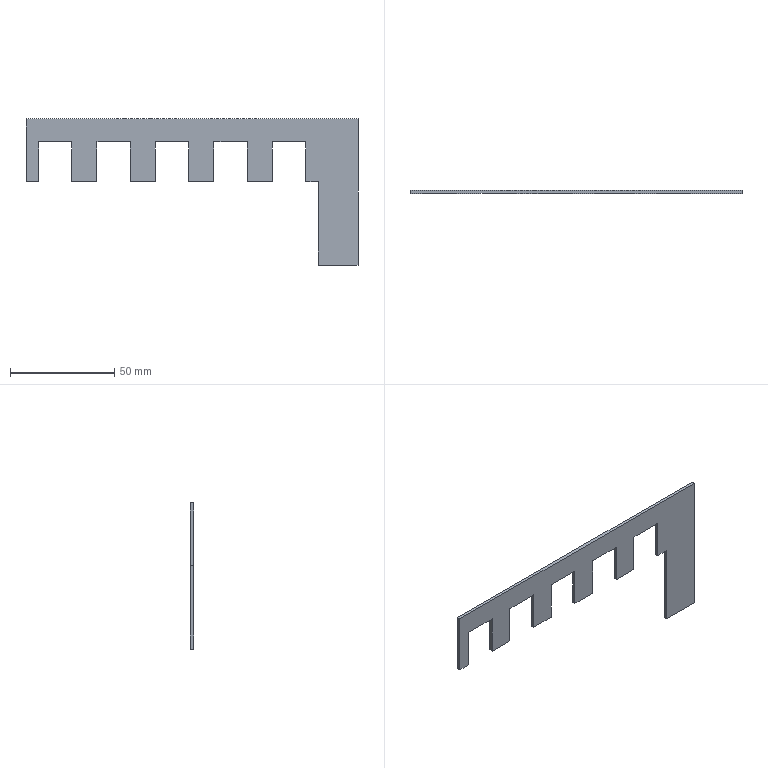Part | STEP file | A14-058 | 1 solid | 28 faces | box 159 x 1.5 x 70 mm | volume 6015 mm3 | plane 28